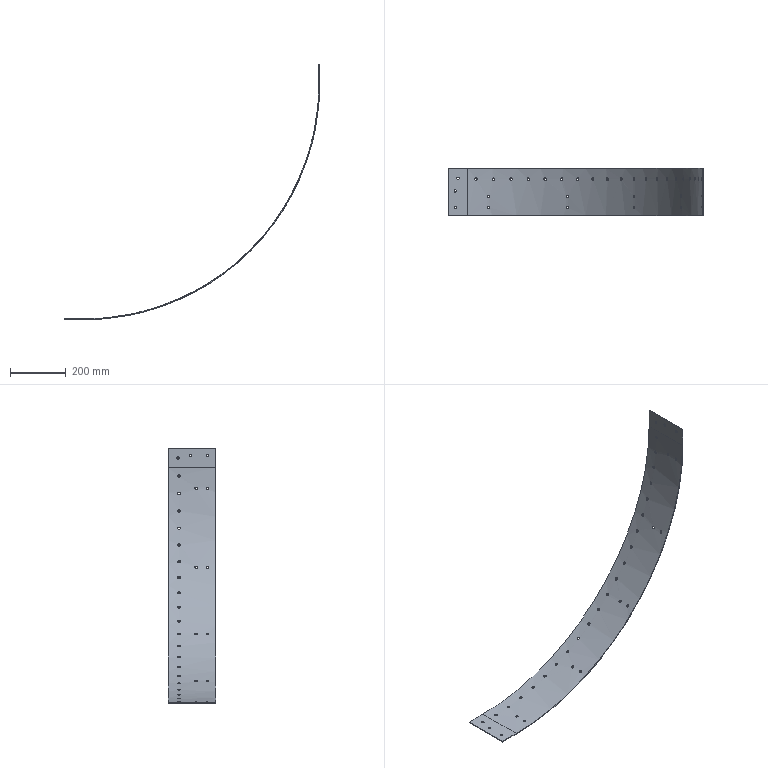Part | STEP file | curverollersinside | 1 solid | 109 faces | box 920 x 170 x 920 mm | volume 620259 mm3 | spline 48 | cone 34 | cylinder 19 | plane 8 | commonest cylinder face diameters 9 x17 1695 x1 1700 x1